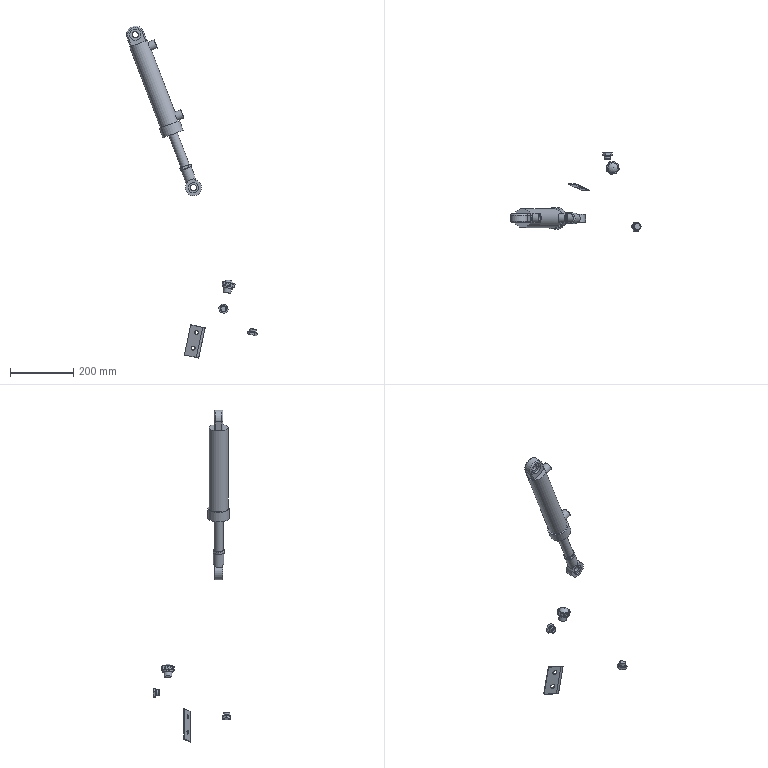Part | STEP file | COMPOUND | 10 solids | 154 faces | box 412.654 x 246 x 1047 mm | volume 1106345 mm3 | cylinder 71 | plane 67 | cone 13 | torus 2 | sphere 1 | commonest cylinder face diameters 8 x20 35 x11 40 x8 20 x4 28 x4 32 x3